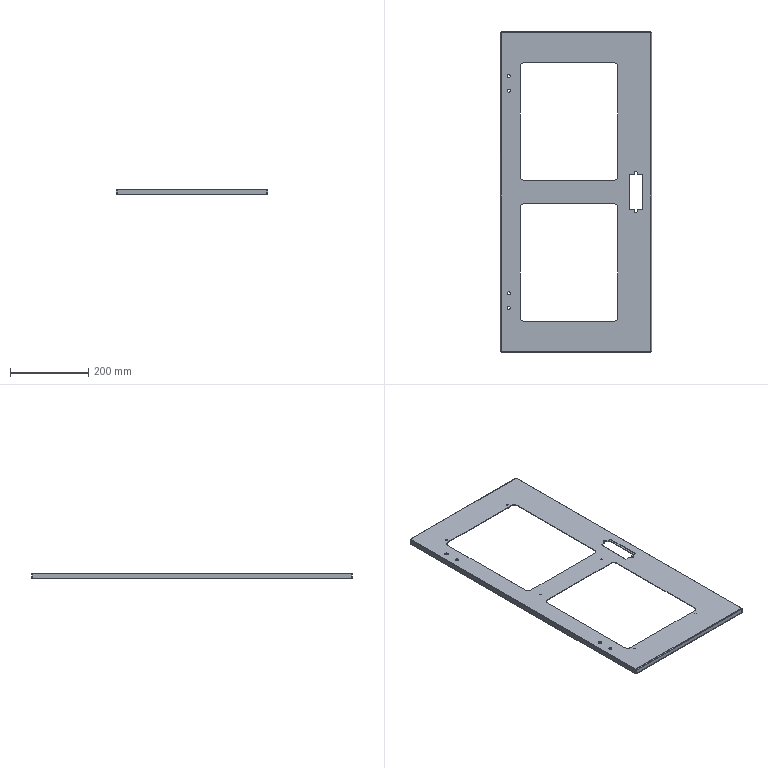Part | STEP file | 09-14 upper door C (Default) | 1 solid | 124 faces | box 386 x 818 x 15 mm | volume 335563 mm3 | plane 62 | cylinder 46 | spline 16 | commonest cylinder face diameters 4 x12 8 x10 1.473 x8 4.473 x8 20 x8